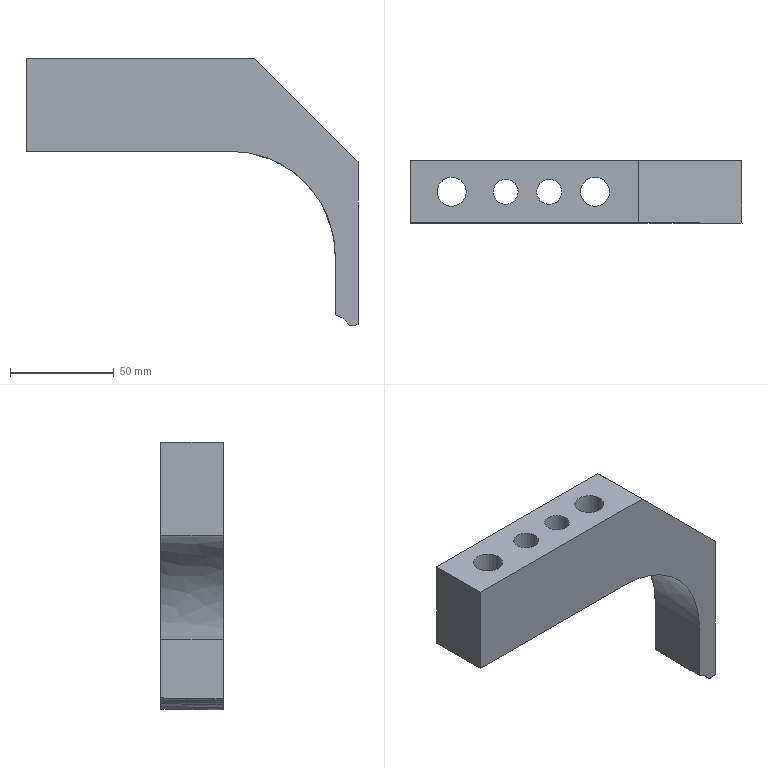Part | NX | features solid 2 | 1 solid | 25 faces | box 160 x 30.001 x 129.104 mm | volume 191101 mm3 | spline 11 | plane 8 | cylinder 6 | commonest cylinder face diameters 12 x2 14 x2 20 x2
STEP:
#1=CARTESIAN_POINT('',(680.804,105.,-27.89));
#2=VERTEX_POINT('',#1);
#3=CARTESIAN_POINT('',(684.074,105.,-28.985));
#4=VERTEX_POINT('',#3);
#5=CARTESIAN_POINT('',(680.804,105.,-27.89));
#6=CARTESIAN_POINT('',(681.537,105.,-28.885));
#7=CARTESIAN_POINT('',(682.89,105.,-29.338));
#8=CARTESIAN_POINT('',(684.074,105.,-28.985));
#9=B_SPLINE_CURVE_WITH_KNOTS('',3,(#5,#6,#7,#8),.UNSPECIFIED.,.F.,.F.,(4,4),(0.,0.003653),.UNSPECIFIED.);
#10=EDGE_CURVE('',#2,#4,#9,.T.);
#11=ORIENTED_EDGE('',*,*,#10,.T.);
#12=CARTESIAN_POINT('',(685.886,105.,-28.443));
#13=VERTEX_POINT('',#12);
#14=CARTESIAN_POINT('',(684.074,105.,-28.985));
#15=CARTESIAN_POINT('',(684.678,105.,-28.805));
#16=CARTESIAN_POINT('',(685.282,105.,-28.624));
#17=CARTESIAN_POINT('',(685.886,105.,-28.443));
#18=B_SPLINE_CURVE_WITH_KNOTS('',3,(#14,#15,#16,#17),.UNSPECIFIED.,.F.,.F.,(4,4),(0.01804,0.01993),.UNSPECIFIED.);
#19=EDGE_CURVE('',#4,#13,#18,.T.);
#20=ORIENTED_EDGE('',*,*,#19,.T.);
#21=CARTESIAN_POINT('',(685.886,105.,50.));
#22=VERTEX_POINT('',#21);
#23=CARTESIAN_POINT('',(685.886,105.,30.));
#24=DIRECTION('',(0.,0.,-1.));
#25=VECTOR('',#24,1000.);
#26=LINE('',#23,#25);
#27=EDGE_CURVE('',#22,#13,#26,.T.);
#28=ORIENTED_EDGE('',*,*,#27,.F.);
#29=CARTESIAN_POINT('',(635.885,105.,100.));
#30=VERTEX_POINT('',#29);
#31=CARTESIAN_POINT('',(685.885,105.,50.));
#32=CARTESIAN_POINT('',(669.219,105.,66.667));
#33=CARTESIAN_POINT('',(652.552,105.,83.333));
#34=CARTESIAN_POINT('',(635.885,105.,100.));
#35=B_SPLINE_CURVE_WITH_KNOTS('',3,(#31,#32,#33,#34),.UNSPECIFIED.,.F.,.F.,(4,4),(0.,1.),.UNSPECIFIED.);
#36=EDGE_CURVE('',#22,#30,#35,.T.);
#37=ORIENTED_EDGE('',*,*,#36,.T.);
#38=CARTESIAN_POINT('',(525.886,105.,100.));
#39=VERTEX_POINT('',#38);
#40=CARTESIAN_POINT('',(664.886,105.,100.));
#41=DIRECTION('',(-1.,0.,0.));
#42=VECTOR('',#41,1000.);
#43=LINE('',#40,#42);
#44=EDGE_CURVE('',#30,#39,#43,.T.);
#45=ORIENTED_EDGE('',*,*,#44,.T.);
#46=CARTESIAN_POINT('',(525.886,105.,55.));
#47=VERTEX_POINT('',#46);
#48=CARTESIAN_POINT('',(525.886,105.,-200.));
#49=DIRECTION('',(0.,0.,1.));
#50=VECTOR('',#49,1000.);
#51=LINE('',#48,#50);
#52=EDGE_CURVE('',#47,#39,#51,.T.);
#53=ORIENTED_EDGE('',*,*,#52,.F.);
#54=CARTESIAN_POINT('',(624.886,105.,55.));
#55=VERTEX_POINT('',#54);
#56=CARTESIAN_POINT('',(531.,105.,55.));
#57=DIRECTION('',(-1.,0.,0.));
#58=VECTOR('',#57,1000.);
#59=LINE('',#56,#58);
#60=EDGE_CURVE('',#55,#47,#59,.T.);
#61=ORIENTED_EDGE('',*,*,#60,.F.);
#62=CARTESIAN_POINT('',(674.886,105.,5.));
#63=VERTEX_POINT('',#62);
#64=CARTESIAN_POINT('',(624.886,105.,55.));
#65=CARTESIAN_POINT('',(628.187,105.,55.));
#66=CARTESIAN_POINT('',(634.66,105.,54.363));
#67=CARTESIAN_POINT('',(644.167,105.,51.481));
#68=CARTESIAN_POINT('',(652.789,105.,46.876));
#69=CARTESIAN_POINT('',(660.473,105.,40.581));
#70=CARTESIAN_POINT('',(666.689,105.,33.01));
#71=CARTESIAN_POINT('',(672.922,105.,21.389));
#72=CARTESIAN_POINT('',(674.886,105.,11.603));
#73=CARTESIAN_POINT('',(674.886,105.,5.));
#74=B_SPLINE_CURVE_WITH_KNOTS('',3,(#64,#65,#66,#67,#68,#69,#70,#71,#72,#73),.UNSPECIFIED.,.F.,.F.,(4,1,1,1,1,1,1,4),(0.,0.009763,0.01953,0.02929,0.03905,0.04882,0.05858,0.07811),.UNSPECIFIED.);
#75=EDGE_CURVE('',#55,#63,#74,.T.);
#76=ORIENTED_EDGE('',*,*,#75,.T.);
#77=CARTESIAN_POINT('',(674.886,105.,-23.672));
#78=VERTEX_POINT('',#77);
#79=CARTESIAN_POINT('',(674.886,105.,44.358));
#80=DIRECTION('',(0.,0.,-1.));
#81=VECTOR('',#80,1000.);
#82=LINE('',#79,#81);
#83=EDGE_CURVE('',#63,#78,#82,.T.);
#84=ORIENTED_EDGE('',*,*,#83,.T.);
#85=CARTESIAN_POINT('',(677.15,105.,-24.654));
#86=VERTEX_POINT('',#85);
#87=CARTESIAN_POINT('',(674.886,105.,-23.672));
#88=CARTESIAN_POINT('',(675.59,105.,-24.088));
#89=CARTESIAN_POINT('',(676.354,105.,-24.42));
#90=CARTESIAN_POINT('',(677.15,105.,-24.654));
#91=B_SPLINE_CURVE_WITH_KNOTS('',3,(#87,#88,#89,#90),.UNSPECIFIED.,.F.,.F.,(4,4),(0.008596,0.01105),.UNSPECIFIED.);
#92=EDGE_CURVE('',#78,#86,#91,.T.);
#93=ORIENTED_EDGE('',*,*,#92,.T.);
#94=CARTESIAN_POINT('',(679.767,105.,-26.484));
#95=VERTEX_POINT('',#94);
#96=CARTESIAN_POINT('',(677.136,105.,-24.65));
#97=CARTESIAN_POINT('',(678.187,105.,-24.955));
#98=CARTESIAN_POINT('',(679.117,105.,-25.604));
#99=CARTESIAN_POINT('',(679.767,105.,-26.484));
#100=B_SPLINE_CURVE_WITH_KNOTS('',3,(#96,#97,#98,#99),.UNSPECIFIED.,.F.,.F.,(4,4),(0.,0.00327),.UNSPECIFIED.);
#101=EDGE_CURVE('',#86,#95,#100,.T.);
#102=ORIENTED_EDGE('',*,*,#101,.T.);
#103=CARTESIAN_POINT('',(679.76,105.,-26.476));
#104=CARTESIAN_POINT('',(680.108,105.,-26.947));
#105=CARTESIAN_POINT('',(680.456,105.,-27.419));
#106=CARTESIAN_POINT('',(680.804,105.,-27.89));
#107=B_SPLINE_CURVE_WITH_KNOTS('',3,(#103,#104,#105,#106),.UNSPECIFIED.,.F.,.F.,(4,4),(0.,0.001758),.UNSPECIFIED.);
#108=EDGE_CURVE('',#95,#2,#107,.T.);
#109=ORIENTED_EDGE('',*,*,#108,.T.);
#110=EDGE_LOOP('',(#11,#20,#28,#37,#45,#53,#61,#76,#84,#93,#102,#109));
#111=FACE_BOUND('',#110,.T.);
#112=CARTESIAN_POINT('',(664.886,105.,-200.));
#113=DIRECTION('',(0.,1.,0.));
#114=DIRECTION('',(0.,0.,1.));
#115=AXIS2_PLACEMENT_3D('',#112,#113,#114);
#116=PLANE('',#115);
#117=ADVANCED_FACE('',(#111),#116,.F.);
#118=CARTESIAN_POINT('',(635.875,135.,100.));
#119=VERTEX_POINT('',#118);
#120=CARTESIAN_POINT('',(525.886,135.,100.));
#121=VERTEX_POINT('',#120);
#122=CARTESIAN_POINT('',(664.883,135.,100.));
#123=DIRECTION('',(-1.,0.,0.));
#124=VECTOR('',#123,1000.);
#125=LINE('',#122,#124);
#126=EDGE_CURVE('',#119,#121,#125,.T.);
#127=ORIENTED_EDGE('',*,*,#126,.F.);
#128=CARTESIAN_POINT('',(685.179,135.,50.704));
#129=VERTEX_POINT('',#128);
#130=CARTESIAN_POINT('',(635.884,135.,100.));
#131=CARTESIAN_POINT('',(652.316,135.,83.568));
#132=CARTESIAN_POINT('',(668.747,135.,67.136));
#133=CARTESIAN_POINT('',(685.179,135.,50.704));
#134=B_SPLINE_CURVE_WITH_KNOTS('',3,(#130,#131,#132,#133),.UNSPECIFIED.,.F.,.F.,(4,4),(0.,1.),.UNSPECIFIED.);
#135=EDGE_CURVE('',#119,#129,#134,.T.);
#136=ORIENTED_EDGE('',*,*,#135,.T.);
#137=CARTESIAN_POINT('',(684.884,135.,30.));
#138=VERTEX_POINT('',#137);
#139=CARTESIAN_POINT('',(685.179,135.,50.704));
#140=CARTESIAN_POINT('',(685.081,135.,43.803));
#141=CARTESIAN_POINT('',(684.982,135.,36.901));
#142=CARTESIAN_POINT('',(684.884,135.,30.));
#143=B_SPLINE_CURVE_WITH_KNOTS('',3,(#139,#140,#141,#142),.UNSPECIFIED.,.F.,.F.,(4,4),(0.7042,1.),.UNSPECIFIED.);
#144=EDGE_CURVE('',#129,#138,#143,.T.);
#145=ORIENTED_EDGE('',*,*,#144,.T.);
#146=CARTESIAN_POINT('',(684.317,135.,30.));
#147=VERTEX_POINT('',#146);
#148=CARTESIAN_POINT('',(684.884,135.,30.));
#149=CARTESIAN_POINT('',(684.695,135.,30.));
#150=CARTESIAN_POINT('',(684.506,135.,30.));
#151=CARTESIAN_POINT('',(684.317,135.,30.));
#152=B_SPLINE_CURVE_WITH_KNOTS('',3,(#148,#149,#150,#151),.UNSPECIFIED.,.F.,.F.,(4,4),(0.,1.),.UNSPECIFIED.);
#153=EDGE_CURVE('',#138,#147,#152,.T.);
#154=ORIENTED_EDGE('',*,*,#153,.T.);
#155=CARTESIAN_POINT('',(674.884,135.001,30.));
#156=VERTEX_POINT('',#155);
#157=CARTESIAN_POINT('',(684.317,135.,30.));
#158=CARTESIAN_POINT('',(681.172,135.,30.));
#159=CARTESIAN_POINT('',(678.028,135.,30.));
#160=CARTESIAN_POINT('',(674.884,135.,30.));
#161=B_SPLINE_CURVE_WITH_KNOTS('',3,(#157,#158,#159,#160),.UNSPECIFIED.,.F.,.F.,(4,4),(0.,1.),.UNSPECIFIED.);
#162=EDGE_CURVE('',#147,#156,#161,.T.);
#163=ORIENTED_EDGE('',*,*,#162,.T.);
#164=CARTESIAN_POINT('',(668.185,135.001,30.));
#165=VERTEX_POINT('',#164);
#166=CARTESIAN_POINT('',(674.884,135.,30.));
#167=CARTESIAN_POINT('',(672.651,135.,30.));
#168=CARTESIAN_POINT('',(670.418,135.,30.));
#169=CARTESIAN_POINT('',(668.185,135.,30.));
#170=B_SPLINE_CURVE_WITH_KNOTS('',3,(#166,#167,#168,#169),.UNSPECIFIED.,.F.,.F.,(4,4),(0.,1.),.UNSPECIFIED.);
#171=EDGE_CURVE('',#156,#165,#170,.T.);
#172=ORIENTED_EDGE('',*,*,#171,.T.);
#173=CARTESIAN_POINT('',(624.884,135.,55.));
#174=VERTEX_POINT('',#173);
#175=CARTESIAN_POINT('',(668.185,135.,30.));
#176=CARTESIAN_POINT('',(665.981,135.,33.818));
#177=CARTESIAN_POINT('',(662.018,135.,38.982));
#178=CARTESIAN_POINT('',(655.372,135.,44.812));
#179=CARTESIAN_POINT('',(649.946,135.,48.428));
#180=CARTESIAN_POINT('',(644.065,135.,51.332));
#181=CARTESIAN_POINT('',(635.725,135.,54.151));
#182=CARTESIAN_POINT('',(629.292,135.,55.));
#183=CARTESIAN_POINT('',(624.884,135.,55.));
#184=B_SPLINE_CURVE_WITH_KNOTS('',3,(#175,#176,#177,#178,#179,#180,#181,#182,#183),.UNSPECIFIED.,.F.,.F.,(4,1,1,1,1,1,4),(0.,0.01304,0.01956,0.02608,0.03259,0.03911,0.05215),.UNSPECIFIED.);
#185=EDGE_CURVE('',#165,#174,#184,.T.);
#186=ORIENTED_EDGE('',*,*,#185,.T.);
#187=CARTESIAN_POINT('',(525.886,135.,55.));
#188=VERTEX_POINT('',#187);
#189=CARTESIAN_POINT('',(664.883,135.,55.));
#190=DIRECTION('',(-1.,0.,0.));
#191=VECTOR('',#190,1000.);
#192=LINE('',#189,#191);
#193=EDGE_CURVE('',#174,#188,#192,.T.);
#194=ORIENTED_EDGE('',*,*,#193,.T.);
#195=CARTESIAN_POINT('',(525.886,135.,-200.));
#196=DIRECTION('',(0.,0.,1.));
#197=VECTOR('',#196,1000.);
#198=LINE('',#195,#197);
#199=EDGE_CURVE('',#188,#121,#198,.T.);
#200=ORIENTED_EDGE('',*,*,#199,.T.);
#201=EDGE_LOOP('',(#127,#136,#145,#154,#163,#172,#186,#194,#200));
#202=FACE_BOUND('',#201,.T.);
#203=CARTESIAN_POINT('',(664.883,135.,-200.));
#204=DIRECTION('',(0.,1.,0.));
#205=DIRECTION('',(0.,0.,1.));
#206=AXIS2_PLACEMENT_3D('',#203,#204,#205);
#207=PLANE('',#206);
#208=ADVANCED_FACE('',(#202),#207,.T.);
#209=CARTESIAN_POINT('',(525.886,135.,55.));
#210=DIRECTION('',(0.,-1.,0.));
#211=VECTOR('',#210,1000.);
#212=LINE('',#209,#211);
#213=EDGE_CURVE('',#188,#47,#212,.T.);
#214=ORIENTED_EDGE('',*,*,#213,.T.);
#215=ORIENTED_EDGE('',*,*,#52,.T.);
#216=CARTESIAN_POINT('',(525.886,175.,100.));
#217=DIRECTION('',(0.,-1.,0.));
#218=VECTOR('',#217,1000.);
#219=LINE('',#216,#218);
#220=EDGE_CURVE('',#121,#39,#219,.T.);
#221=ORIENTED_EDGE('',*,*,#220,.F.);
#222=ORIENTED_EDGE('',*,*,#199,.F.);
#223=EDGE_LOOP('',(#214,#215,#221,#222));
#224=FACE_BOUND('',#223,.T.);
#225=CARTESIAN_POINT('',(525.886,175.,75.));
#226=DIRECTION('',(-1.,0.,0.));
#227=DIRECTION('',(0.,0.,1.));
#228=AXIS2_PLACEMENT_3D('',#225,#226,#227);
#229=PLANE('',#228);
#230=ADVANCED_FACE('',(#224),#229,.T.);
#231=CARTESIAN_POINT('',(587.,120.,100.));
#232=VERTEX_POINT('',#231);
#233=CARTESIAN_POINT('',(593.,120.,100.));
#234=DIRECTION('',(0.,0.,-1.));
#235=DIRECTION('',(-1.,0.,0.));
#236=AXIS2_PLACEMENT_3D('',#233,#234,#235);
#237=CIRCLE('',#236,6.);
#238=EDGE_CURVE('',#232,#232,#237,.T.);
#239=ORIENTED_EDGE('',*,*,#238,.T.);
#240=EDGE_LOOP('',(#239));
#241=FACE_BOUND('',#240,.T.);
#242=CARTESIAN_POINT('',(566.,120.,100.));
#243=VERTEX_POINT('',#242);
#244=CARTESIAN_POINT('',(572.,120.,100.));
#245=DIRECTION('',(0.,0.,-1.));
#246=DIRECTION('',(-1.,0.,0.));
#247=AXIS2_PLACEMENT_3D('',#244,#245,#246);
#248=CIRCLE('',#247,6.);
#249=EDGE_CURVE('',#243,#243,#248,.T.);
#250=ORIENTED_EDGE('',*,*,#249,.T.);
#251=EDGE_LOOP('',(#250));
#252=FACE_BOUND('',#251,.T.);
#253=CARTESIAN_POINT('',(608.,120.,100.));
#254=VERTEX_POINT('',#253);
#255=CARTESIAN_POINT('',(615.,120.,100.));
#256=DIRECTION('',(0.,0.,-1.));
#257=DIRECTION('',(-1.,0.,0.));
#258=AXIS2_PLACEMENT_3D('',#255,#256,#257);
#259=CIRCLE('',#258,7.);
#260=EDGE_CURVE('',#254,#254,#259,.T.);
#261=ORIENTED_EDGE('',*,*,#260,.T.);
#262=EDGE_LOOP('',(#261));
#263=FACE_BOUND('',#262,.T.);
#264=CARTESIAN_POINT('',(539.,120.,100.));
#265=VERTEX_POINT('',#264);
#266=CARTESIAN_POINT('',(546.,120.,100.));
#267=DIRECTION('',(0.,0.,-1.));
#268=DIRECTION('',(-1.,0.,0.));
#269=AXIS2_PLACEMENT_3D('',#266,#267,#268);
#270=CIRCLE('',#269,7.);
#271=EDGE_CURVE('',#265,#265,#270,.T.);
#272=ORIENTED_EDGE('',*,*,#271,.T.);
#273=EDGE_LOOP('',(#272));
#274=FACE_BOUND('',#273,.T.);
#275=ORIENTED_EDGE('',*,*,#44,.F.);
#276=CARTESIAN_POINT('',(635.885,105.,100.));
#277=CARTESIAN_POINT('',(635.885,115.,100.));
#278=CARTESIAN_POINT('',(635.884,125.,100.));
#279=CARTESIAN_POINT('',(635.884,135.,100.));
#280=B_SPLINE_CURVE_WITH_KNOTS('',3,(#276,#277,#278,#279),.UNSPECIFIED.,.F.,.F.,(4,4),(0.,1.),.UNSPECIFIED.);
#281=EDGE_CURVE('',#30,#119,#280,.T.);
#282=ORIENTED_EDGE('',*,*,#281,.T.);
#283=ORIENTED_EDGE('',*,*,#126,.T.);
#284=ORIENTED_EDGE('',*,*,#220,.T.);
#285=EDGE_LOOP('',(#275,#282,#283,#284));
#286=FACE_BOUND('',#285,.T.);
#287=CARTESIAN_POINT('',(561.,60.,100.));
#288=DIRECTION('',(0.,0.,-1.));
#289=DIRECTION('',(-1.,0.,0.));
#290=AXIS2_PLACEMENT_3D('',#287,#288,#289);
#291=PLANE('',#290);
#292=ADVANCED_FACE('',(#241,#252,#263,#274,#286),#291,.F.);
#293=CARTESIAN_POINT('',(553.,120.,75.));
#294=VERTEX_POINT('',#293);
#295=CARTESIAN_POINT('',(546.,120.,75.));
#296=DIRECTION('',(0.,0.,1.));
#297=DIRECTION('',(1.,0.,0.));
#298=AXIS2_PLACEMENT_3D('',#295,#296,#297);
#299=CIRCLE('',#298,7.);
#300=EDGE_CURVE('',#294,#294,#299,.T.);
#301=ORIENTED_EDGE('',*,*,#300,.F.);
#302=EDGE_LOOP('',(#301));
#303=FACE_BOUND('',#302,.T.);
#304=ORIENTED_EDGE('',*,*,#271,.F.);
#305=EDGE_LOOP('',(#304));
#306=FACE_BOUND('',#305,.T.);
#307=CARTESIAN_POINT('',(546.,120.,75.));
#308=DIRECTION('',(0.,0.,1.));
#309=DIRECTION('',(-1.,0.,0.));
#310=AXIS2_PLACEMENT_3D('',#307,#308,#309);
#311=CYLINDRICAL_SURFACE('',#310,7.);
#312=ADVANCED_FACE('',(#303,#306),#311,.F.);
#313=ORIENTED_EDGE('',*,*,#300,.T.);
#314=EDGE_LOOP('',(#313));
#315=FACE_BOUND('',#314,.T.);
#316=CARTESIAN_POINT('',(556.,120.,75.));
#317=VERTEX_POINT('',#316);
#318=CARTESIAN_POINT('',(546.,120.,75.));
#319=DIRECTION('',(0.,0.,-1.));
#320=DIRECTION('',(1.,0.,0.));
#321=AXIS2_PLACEMENT_3D('',#318,#319,#320);
#322=CIRCLE('',#321,10.);
#323=EDGE_CURVE('',#317,#317,#322,.T.);
#324=ORIENTED_EDGE('',*,*,#323,.T.);
#325=EDGE_LOOP('',(#324));
#326=FACE_BOUND('',#325,.T.);
#327=CARTESIAN_POINT('',(546.,120.,75.));
#328=DIRECTION('',(0.,0.,1.));
#329=DIRECTION('',(-1.,0.,0.));
#330=AXIS2_PLACEMENT_3D('',#327,#328,#329);
#331=PLANE('',#330);
#332=ADVANCED_FACE('',(#315,#326),#331,.F.);
#333=CARTESIAN_POINT('',(556.,120.,55.));
#334=VERTEX_POINT('',#333);
#335=CARTESIAN_POINT('',(546.,120.,55.));
#336=DIRECTION('',(0.,0.,1.));
#337=DIRECTION('',(1.,0.,0.));
#338=AXIS2_PLACEMENT_3D('',#335,#336,#337);
#339=CIRCLE('',#338,10.);
#340=EDGE_CURVE('',#334,#334,#339,.F.);
#341=ORIENTED_EDGE('',*,*,#340,.T.);
#342=EDGE_LOOP('',(#341));
#343=FACE_BOUND('',#342,.T.);
#344=ORIENTED_EDGE('',*,*,#323,.F.);
#345=EDGE_LOOP('',(#344));
#346=FACE_BOUND('',#345,.T.);
#347=CARTESIAN_POINT('',(546.,120.,75.));
#348=DIRECTION('',(0.,0.,-1.));
#349=DIRECTION('',(1.,0.,0.));
#350=AXIS2_PLACEMENT_3D('',#347,#348,#349);
#351=CYLINDRICAL_SURFACE('',#350,10.);
#352=ADVANCED_FACE('',(#343,#346),#351,.F.);
#353=CARTESIAN_POINT('',(622.,120.,75.));
#354=VERTEX_POINT('',#353);
#355=CARTESIAN_POINT('',(615.,120.,75.));
#356=DIRECTION('',(0.,0.,1.));
#357=DIRECTION('',(1.,0.,0.));
#358=AXIS2_PLACEMENT_3D('',#355,#356,#357);
#359=CIRCLE('',#358,7.);
#360=EDGE_CURVE('',#354,#354,#359,.T.);
#361=ORIENTED_EDGE('',*,*,#360,.F.);
#362=EDGE_LOOP('',(#361));
#363=FACE_BOUND('',#362,.T.);
#364=ORIENTED_EDGE('',*,*,#260,.F.);
#365=EDGE_LOOP('',(#364));
#366=FACE_BOUND('',#365,.T.);
#367=CARTESIAN_POINT('',(615.,120.,72.));
#368=DIRECTION('',(0.,0.,1.));
#369=DIRECTION('',(-1.,0.,0.));
#370=AXIS2_PLACEMENT_3D('',#367,#368,#369);
#371=CYLINDRICAL_SURFACE('',#370,7.);
#372=ADVANCED_FACE('',(#363,#366),#371,.F.);
#373=CARTESIAN_POINT('',(624.883,118.475,55.));
#374=VERTEX_POINT('',#373);
#375=CARTESIAN_POINT('',(624.883,121.526,55.));
#376=VERTEX_POINT('',#375);
#377=CARTESIAN_POINT('',(615.,120.,55.));
#378=DIRECTION('',(0.,0.,1.));
#379=DIRECTION('',(1.,0.,0.));
#380=AXIS2_PLACEMENT_3D('',#377,#378,#379);
#381=CIRCLE('',#380,10.);
#382=EDGE_CURVE('',#374,#376,#381,.F.);
#383=ORIENTED_EDGE('',*,*,#382,.T.);
#384=CARTESIAN_POINT('',(624.883,118.475,55.));
#385=CARTESIAN_POINT('',(625.038,119.479,55.));
#386=CARTESIAN_POINT('',(625.038,120.522,55.));
#387=CARTESIAN_POINT('',(624.883,121.526,55.));
#388=B_SPLINE_CURVE_WITH_KNOTS('',3,(#384,#385,#386,#387),.UNSPECIFIED.,.F.,.F.,(4,4),(0.001833,0.00488),.UNSPECIFIED.);
#389=EDGE_CURVE('',#376,#374,#388,.F.);
#390=ORIENTED_EDGE('',*,*,#389,.T.);
#391=EDGE_LOOP('',(#383,#390));
#392=FACE_BOUND('',#391,.T.);
#393=CARTESIAN_POINT('',(625.,120.,75.));
#394=VERTEX_POINT('',#393);
#395=CARTESIAN_POINT('',(615.,120.,75.));
#396=DIRECTION('',(0.,0.,1.));
#397=DIRECTION('',(1.,0.,0.));
#398=AXIS2_PLACEMENT_3D('',#395,#396,#397);
#399=CIRCLE('',#398,10.);
#400=EDGE_CURVE('',#394,#394,#399,.F.);
#401=ORIENTED_EDGE('',*,*,#400,.F.);
#402=EDGE_LOOP('',(#401));
#403=FACE_BOUND('',#402,.T.);
#404=CARTESIAN_POINT('',(615.,120.,72.));
#405=DIRECTION('',(0.,0.,-1.));
#406=DIRECTION('',(1.,0.,0.));
#407=AXIS2_PLACEMENT_3D('',#404,#405,#406);
#408=CYLINDRICAL_SURFACE('',#407,10.);
#409=ADVANCED_FACE('',(#392,#403),#408,.F.);
#410=ORIENTED_EDGE('',*,*,#360,.T.);
#411=EDGE_LOOP('',(#410));
#412=FACE_BOUND('',#411,.T.);
#413=ORIENTED_EDGE('',*,*,#400,.T.);
#414=EDGE_LOOP('',(#413));
#415=FACE_BOUND('',#414,.T.);
#416=CARTESIAN_POINT('',(615.,120.,75.));
#417=DIRECTION('',(0.,0.,1.));
#418=DIRECTION('',(-1.,0.,0.));
#419=AXIS2_PLACEMENT_3D('',#416,#417,#418);
#420=PLANE('',#419);
#421=ADVANCED_FACE('',(#412,#415),#420,.F.);
#422=CARTESIAN_POINT('',(587.,120.,55.));
#423=VERTEX_POINT('',#422);
#424=CARTESIAN_POINT('',(593.,120.,55.));
#425=DIRECTION('',(0.,0.,-1.));
#426=DIRECTION('',(-1.,0.,0.));
#427=AXIS2_PLACEMENT_3D('',#424,#425,#426);
#428=CIRCLE('',#427,6.);
#429=EDGE_CURVE('',#423,#423,#428,.T.);
#430=ORIENTED_EDGE('',*,*,#429,.F.);
#431=EDGE_LOOP('',(#430));
#432=FACE_BOUND('',#431,.T.);
#433=CARTESIAN_POINT('',(566.,120.,55.));
#434=VERTEX_POINT('',#433);
#435=CARTESIAN_POINT('',(572.,120.,55.));
#436=DIRECTION('',(0.,0.,-1.));
#437=DIRECTION('',(-1.,0.,0.));
#438=AXIS2_PLACEMENT_3D('',#435,#436,#437);
#439=CIRCLE('',#438,6.);
#440=EDGE_CURVE('',#434,#434,#439,.T.);
#441=ORIENTED_EDGE('',*,*,#440,.F.);
#442=EDGE_LOOP('',(#441));
#443=FACE_BOUND('',#442,.T.);
#444=ORIENTED_EDGE('',*,*,#193,.F.);
#445=CARTESIAN_POINT('',(624.884,135.,55.));
#446=CARTESIAN_POINT('',(624.883,130.509,55.));
#447=CARTESIAN_POINT('',(624.883,126.017,55.));
#448=CARTESIAN_POINT('',(624.883,121.526,55.));
#449=B_SPLINE_CURVE_WITH_KNOTS('',3,(#445,#446,#447,#448),.UNSPECIFIED.,.F.,.F.,(4,4),(0.,0.01347),.UNSPECIFIED.);
#450=EDGE_CURVE('',#174,#376,#449,.T.);
#451=ORIENTED_EDGE('',*,*,#450,.T.);
#452=ORIENTED_EDGE('',*,*,#382,.F.);
#453=CARTESIAN_POINT('',(624.883,118.475,55.));
#454=CARTESIAN_POINT('',(624.883,113.983,55.));
#455=CARTESIAN_POINT('',(624.884,109.492,55.));
#456=CARTESIAN_POINT('',(624.886,105.,55.));
#457=B_SPLINE_CURVE_WITH_KNOTS('',3,(#453,#454,#455,#456),.UNSPECIFIED.,.F.,.F.,(4,4),(0.01653,0.03),.UNSPECIFIED.);
#458=EDGE_CURVE('',#374,#55,#457,.T.);
#459=ORIENTED_EDGE('',*,*,#458,.T.);
#460=ORIENTED_EDGE('',*,*,#60,.T.);
#461=ORIENTED_EDGE('',*,*,#213,.F.);
#462=EDGE_LOOP('',(#444,#451,#452,#459,#460,#461));
#463=FACE_BOUND('',#462,.T.);
#464=ORIENTED_EDGE('',*,*,#340,.F.);
#465=EDGE_LOOP('',(#464));
#466=FACE_BOUND('',#465,.T.);
#467=CARTESIAN_POINT('',(531.,135.,55.));
#468=DIRECTION('',(0.,0.,1.));
#469=DIRECTION('',(0.,-1.,0.));
#470=AXIS2_PLACEMENT_3D('',#467,#468,#469);
#471=PLANE('',#470);
#472=ADVANCED_FACE('',(#432,#443,#463,#466),#471,.F.);
#473=ORIENTED_EDGE('',*,*,#249,.F.);
#474=EDGE_LOOP('',(#473));
#475=FACE_BOUND('',#474,.T.);
#476=ORIENTED_EDGE('',*,*,#440,.T.);
#477=EDGE_LOOP('',(#476));
#478=FACE_BOUND('',#477,.T.);
#479=CARTESIAN_POINT('',(572.,120.,105.));
#480=DIRECTION('',(0.,0.,-1.));
#481=DIRECTION('',(-1.,0.,0.));
#482=AXIS2_PLACEMENT_3D('',#479,#480,#481);
#483=CYLINDRICAL_SURFACE('',#482,6.);
#484=ADVANCED_FACE('',(#475,#478),#483,.F.);
#485=ORIENTED_EDGE('',*,*,#238,.F.);
#486=EDGE_LOOP('',(#485));
#487=FACE_BOUND('',#486,.T.);
#488=ORIENTED_EDGE('',*,*,#429,.T.);
#489=EDGE_LOOP('',(#488));
#490=FACE_BOUND('',#489,.T.);
#491=CARTESIAN_POINT('',(593.,120.,105.));
#492=DIRECTION('',(0.,0.,-1.));
#493=DIRECTION('',(-1.,0.,0.));
#494=AXIS2_PLACEMENT_3D('',#491,#492,#493);
#495=CYLINDRICAL_SURFACE('',#494,6.);
#496=ADVANCED_FACE('',(#487,#490),#495,.F.);
#497=CARTESIAN_POINT('',(674.884,135.001,-23.321));
#498=VERTEX_POINT('',#497);
#499=CARTESIAN_POINT('',(674.883,122.627,-23.464));
#500=VERTEX_POINT('',#499);
#501=CARTESIAN_POINT('',(674.884,135.001,-23.321));
#502=CARTESIAN_POINT('',(674.883,130.876,-23.369));
#503=CARTESIAN_POINT('',(674.883,126.752,-23.415));
#504=CARTESIAN_POINT('',(674.883,122.627,-23.464));
#505=B_SPLINE_CURVE_WITH_KNOTS('',3,(#501,#502,#503,#504),.UNSPECIFIED.,.F.,.F.,(4,4),(0.,0.01237),.UNSPECIFIED.);
#506=EDGE_CURVE('',#498,#500,#505,.T.);
#507=ORIENTED_EDGE('',*,*,#506,.T.);
#508=CARTESIAN_POINT('',(674.883,122.627,-23.464));
#509=CARTESIAN_POINT('',(674.883,116.751,-23.533));
#510=CARTESIAN_POINT('',(674.884,110.876,-23.603));
#511=CARTESIAN_POINT('',(674.886,105.,-23.672));
#512=B_SPLINE_CURVE_WITH_KNOTS('',3,(#508,#509,#510,#511),.UNSPECIFIED.,.F.,.F.,(4,4),(0.,0.01763),.UNSPECIFIED.);
#513=EDGE_CURVE('',#500,#78,#512,.T.);
#514=ORIENTED_EDGE('',*,*,#513,.T.);
#515=ORIENTED_EDGE('',*,*,#83,.F.);
#516=CARTESIAN_POINT('',(674.884,135.001,5.));
#517=VERTEX_POINT('',#516);
#518=CARTESIAN_POINT('',(674.886,105.,5.));
#519=CARTESIAN_POINT('',(674.882,115.,5.));
#520=CARTESIAN_POINT('',(674.883,125.001,5.));
#521=CARTESIAN_POINT('',(674.884,135.001,5.));
#522=B_SPLINE_CURVE_WITH_KNOTS('',3,(#518,#519,#520,#521),.UNSPECIFIED.,.F.,.F.,(4,4),(0.,0.03),.UNSPECIFIED.);
#523=EDGE_CURVE('',#63,#517,#522,.T.);
#524=ORIENTED_EDGE('',*,*,#523,.T.);
#525=CARTESIAN_POINT('',(674.884,135.001,30.));
#526=DIRECTION('',(0.,0.,-1.));
#527=VECTOR('',#526,1000.);
#528=LINE('',#525,#527);
#529=EDGE_CURVE('',#517,#498,#528,.T.);
#530=ORIENTED_EDGE('',*,*,#529,.T.);
#531=EDGE_LOOP('',(#507,#514,#515,#524,#530));
#532=FACE_BOUND('',#531,.T.);
#533=CARTESIAN_POINT('',(674.884,135.001,5.));
#534=CARTESIAN_POINT('',(674.884,135.001,-23.844));
#535=CARTESIAN_POINT('',(674.883,125.002,5.));
#536=CARTESIAN_POINT('',(674.883,125.002,-23.844));
#537=CARTESIAN_POINT('',(674.882,115.001,5.));
#538=CARTESIAN_POINT('',(674.882,115.001,-23.844));
#539=CARTESIAN_POINT('',(674.886,105.,5.));
#540=CARTESIAN_POINT('',(674.886,105.,-23.844));
#541=B_SPLINE_SURFACE_WITH_KNOTS('',3,1,((#533,#534),(#535,#536),(#537,#538),(#539,#540)),.SURF_OF_LINEAR_EXTRUSION.,.F.,.F.,.F.,(4,4),(2,2),(0.,0.9999),(0.,1.),.PIECEWISE_BEZIER_KNOTS.);
#542=ADVANCED_FACE('',(#532),#541,.F.);
#543=CARTESIAN_POINT('',(684.075,135.,-28.612));
#544=VERTEX_POINT('',#543);
#545=CARTESIAN_POINT('',(685.884,135.,-28.07));
#546=VERTEX_POINT('',#545);
#547=CARTESIAN_POINT('',(684.075,135.,-28.612));
#548=CARTESIAN_POINT('',(684.678,135.,-28.432));
#549=CARTESIAN_POINT('',(685.281,135.,-28.251));
#550=CARTESIAN_POINT('',(685.884,135.,-28.07));
#551=B_SPLINE_CURVE_WITH_KNOTS('',3,(#547,#548,#549,#550),.UNSPECIFIED.,.F.,.F.,(4,4),(0.01663,0.01852),.UNSPECIFIED.);
#552=EDGE_CURVE('',#544,#546,#551,.T.);
#553=ORIENTED_EDGE('',*,*,#552,.F.);
#554=CARTESIAN_POINT('',(680.804,135.,-27.517));
#555=VERTEX_POINT('',#554);
#556=CARTESIAN_POINT('',(680.804,135.,-27.517));
#557=CARTESIAN_POINT('',(681.537,135.,-28.511));
#558=CARTESIAN_POINT('',(682.891,135.,-28.964));
#559=CARTESIAN_POINT('',(684.074,135.,-28.612));
#560=B_SPLINE_CURVE_WITH_KNOTS('',3,(#556,#557,#558,#559),.UNSPECIFIED.,.F.,.F.,(4,4),(0.,0.003653),.UNSPECIFIED.);
#561=EDGE_CURVE('',#555,#544,#560,.T.);
#562=ORIENTED_EDGE('',*,*,#561,.F.);
#563=CARTESIAN_POINT('',(679.774,135.,-26.121));
#564=VERTEX_POINT('',#563);
#565=CARTESIAN_POINT('',(679.776,135.,-26.124));
#566=CARTESIAN_POINT('',(680.119,135.,-26.588));
#567=CARTESIAN_POINT('',(680.461,135.,-27.053));
#568=CARTESIAN_POINT('',(680.804,135.,-27.517));
#569=B_SPLINE_CURVE_WITH_KNOTS('',3,(#565,#566,#567,#568),.UNSPECIFIED.,.F.,.F.,(4,4),(0.00002659,0.001758),.UNSPECIFIED.);
#570=EDGE_CURVE('',#564,#555,#569,.T.);
#571=ORIENTED_EDGE('',*,*,#570,.F.);
#572=CARTESIAN_POINT('',(677.142,135.001,-24.284));
#573=VERTEX_POINT('',#572);
#574=CARTESIAN_POINT('',(677.149,135.001,-24.286));
#575=CARTESIAN_POINT('',(678.198,135.001,-24.593));
#576=CARTESIAN_POINT('',(679.122,135.001,-25.236));
#577=CARTESIAN_POINT('',(679.772,135.,-26.118));
#578=B_SPLINE_CURVE_WITH_KNOTS('',3,(#574,#575,#576,#577),.UNSPECIFIED.,.F.,.F.,(4,4),(0.001293,0.004557),.UNSPECIFIED.);
#579=EDGE_CURVE('',#573,#564,#578,.T.);
#580=ORIENTED_EDGE('',*,*,#579,.F.);
#581=CARTESIAN_POINT('',(674.884,135.001,-23.321));
#582=CARTESIAN_POINT('',(675.585,135.001,-23.728));
#583=CARTESIAN_POINT('',(676.345,135.001,-24.054));
#584=CARTESIAN_POINT('',(677.135,135.001,-24.282));
#585=B_SPLINE_CURVE_WITH_KNOTS('',3,(#581,#582,#583,#584),.UNSPECIFIED.,.F.,.F.,(4,4),(0.008683,0.01112),.UNSPECIFIED.);
#586=EDGE_CURVE('',#498,#573,#585,.T.);
#587=ORIENTED_EDGE('',*,*,#586,.F.);
#588=ORIENTED_EDGE('',*,*,#529,.F.);
#589=CARTESIAN_POINT('',(624.884,135.005,5.));
#590=DIRECTION('',(-0.00008819,-1.,0.));
#591=DIRECTION('',(1.,-0.00008819,0.));
#592=AXIS2_PLACEMENT_3D('',#589,#590,#591);
#593=CIRCLE('',#592,50.);
#594=EDGE_CURVE('',#517,#165,#593,.T.);
#595=ORIENTED_EDGE('',*,*,#594,.T.);
#596=ORIENTED_EDGE('',*,*,#171,.F.);
#597=ORIENTED_EDGE('',*,*,#162,.F.);
#598=ORIENTED_EDGE('',*,*,#153,.F.);
#599=ORIENTED_EDGE('',*,*,#144,.F.);
#600=CARTESIAN_POINT('',(685.884,135.,50.));
#601=VERTEX_POINT('',#600);
#602=CARTESIAN_POINT('',(685.179,135.,50.704));
#603=CARTESIAN_POINT('',(685.414,135.,50.469));
#604=CARTESIAN_POINT('',(685.649,135.,50.235));
#605=CARTESIAN_POINT('',(685.884,135.,50.));
#606=B_SPLINE_CURVE_WITH_KNOTS('',3,(#602,#603,#604,#605),.UNSPECIFIED.,.F.,.F.,(4,4),(0.,1.),.UNSPECIFIED.);
#607=EDGE_CURVE('',#129,#601,#606,.T.);
#608=ORIENTED_EDGE('',*,*,#607,.T.);
#609=CARTESIAN_POINT('',(685.884,135.,30.));
#610=DIRECTION('',(0.,0.,-1.));
#611=VECTOR('',#610,1000.);
#612=LINE('',#609,#611);
#613=EDGE_CURVE('',#601,#546,#612,.T.);
#614=ORIENTED_EDGE('',*,*,#613,.T.);
#615=EDGE_LOOP('',(#553,#562,#571,#580,#587,#588,#595,#596,#597,#598,#599,#608,#614));
#616=FACE_BOUND('',#615,.T.);
#617=CARTESIAN_POINT('',(684.884,135.,30.));
#618=DIRECTION('',(-0.00008819,-1.,0.));
#619=DIRECTION('',(0.,0.,-1.));
#620=AXIS2_PLACEMENT_3D('',#617,#618,#619);
#621=PLANE('',#620);
#622=ADVANCED_FACE('',(#616),#621,.F.);
#623=CARTESIAN_POINT('',(685.884,135.,-28.07));
#624=CARTESIAN_POINT('',(685.883,125.,-28.196));
#625=CARTESIAN_POINT('',(685.882,115.,-28.32));
#626=CARTESIAN_POINT('',(685.886,105.,-28.443));
#627=B_SPLINE_CURVE_WITH_KNOTS('',3,(#623,#624,#625,#626),.UNSPECIFIED.,.F.,.F.,(4,4),(0.,0.03),.UNSPECIFIED.);
#628=EDGE_CURVE('',#546,#13,#627,.T.);
#629=ORIENTED_EDGE('',*,*,#628,.F.);
#630=ORIENTED_EDGE('',*,*,#613,.F.);
#631=CARTESIAN_POINT('',(685.885,105.,50.));
#632=CARTESIAN_POINT('',(685.882,114.999,50.));
#633=CARTESIAN_POINT('',(685.883,124.992,50.));
#634=CARTESIAN_POINT('',(685.884,135.,50.));
#635=B_SPLINE_CURVE_WITH_KNOTS('',3,(#631,#632,#633,#634),.UNSPECIFIED.,.F.,.F.,(4,4),(0.,1.),.UNSPECIFIED.);
#636=EDGE_CURVE('',#601,#22,#635,.F.);
#637=ORIENTED_EDGE('',*,*,#636,.T.);
#638=ORIENTED_EDGE('',*,*,#27,.T.);
#639=EDGE_LOOP('',(#629,#630,#637,#638));
#640=FACE_BOUND('',#639,.T.);
#641=CARTESIAN_POINT('',(685.884,135.,50.));
#642=CARTESIAN_POINT('',(685.884,135.,-28.913));
#643=CARTESIAN_POINT('',(685.883,125.,50.));
#644=CARTESIAN_POINT('',(685.883,125.,-28.913));
#645=CARTESIAN_POINT('',(685.882,115.,50.));
#646=CARTESIAN_POINT('',(685.882,115.,-28.913));
#647=CARTESIAN_POINT('',(685.886,105.,50.));
#648=CARTESIAN_POINT('',(685.886,105.,-28.913));
#649=B_SPLINE_SURFACE_WITH_KNOTS('',3,1,((#641,#642),(#643,#644),(#645,#646),(#647,#648)),.SURF_OF_LINEAR_EXTRUSION.,.F.,.F.,.F.,(4,4),(2,2),(0.,1.),(0.,1.),.PIECEWISE_BEZIER_KNOTS.);
#650=ADVANCED_FACE('',(#640),#649,.T.);
#651=ORIENTED_EDGE('',*,*,#594,.F.);
#652=ORIENTED_EDGE('',*,*,#523,.F.);
#653=ORIENTED_EDGE('',*,*,#75,.F.);
#654=ORIENTED_EDGE('',*,*,#458,.F.);
#655=ORIENTED_EDGE('',*,*,#389,.F.);
#656=ORIENTED_EDGE('',*,*,#450,.F.);
#657=ORIENTED_EDGE('',*,*,#185,.F.);
#658=EDGE_LOOP('',(#651,#652,#653,#654,#655,#656,#657));
#659=FACE_BOUND('',#658,.T.);
#660=CARTESIAN_POINT('',(624.884,135.005,55.));
#661=CARTESIAN_POINT('',(674.884,135.001,55.));
#662=CARTESIAN_POINT('',(674.884,135.001,5.));
#663=CARTESIAN_POINT('',(624.883,124.938,55.));
#664=CARTESIAN_POINT('',(674.883,124.932,55.));
#665=CARTESIAN_POINT('',(674.883,124.932,5.));
#666=CARTESIAN_POINT('',(624.882,114.871,55.));
#667=CARTESIAN_POINT('',(674.882,114.887,55.));
#668=CARTESIAN_POINT('',(674.882,114.887,5.));
#669=CARTESIAN_POINT('',(624.886,104.804,55.));
#670=CARTESIAN_POINT('',(674.886,104.82,55.));
#671=CARTESIAN_POINT('',(674.886,104.82,5.));
#672=(BOUNDED_SURFACE()B_SPLINE_SURFACE(3,2,((#660,#661,#662),(#663,#664,#665),(#666,#667,#668),(#669,#670,#671)),.UNSPECIFIED.,.F.,.F.,.F.)B_SPLINE_SURFACE_WITH_KNOTS((4,4),(3,3),(0.12,0.1502),(0.,1.),.PIECEWISE_BEZIER_KNOTS.)GEOMETRIC_REPRESENTATION_ITEM()RATIONAL_B_SPLINE_SURFACE(((1.,0.7071,1.),(1.,0.7071,1.),(1.,0.7071,1.),(1.,0.7071,1.)))REPRESENTATION_ITEM('')SURFACE());
#673=ADVANCED_FACE('',(#659),#672,.F.);
#674=ORIENTED_EDGE('',*,*,#135,.F.);
#675=ORIENTED_EDGE('',*,*,#281,.F.);
#676=ORIENTED_EDGE('',*,*,#36,.F.);
#677=ORIENTED_EDGE('',*,*,#636,.F.);
#678=ORIENTED_EDGE('',*,*,#607,.F.);
#679=EDGE_LOOP('',(#674,#675,#676,#677,#678));
#680=FACE_BOUND('',#679,.T.);
#681=CARTESIAN_POINT('',(635.886,104.805,100.));
#682=CARTESIAN_POINT('',(635.882,114.871,100.));
#683=CARTESIAN_POINT('',(635.883,124.938,100.));
#684=CARTESIAN_POINT('',(635.884,135.005,100.));
#685=CARTESIAN_POINT('',(685.886,104.82,50.));
#686=CARTESIAN_POINT('',(685.882,114.879,50.));
#687=CARTESIAN_POINT('',(685.883,124.932,50.));
#688=CARTESIAN_POINT('',(685.884,135.,50.));
#689=B_SPLINE_SURFACE_WITH_KNOTS('',1,3,((#681,#682,#683,#684),(#685,#686,#687,#688)),.RULED_SURF.,.F.,.F.,.F.,(2,2),(4,4),(0.,1.),(0.1225,0.1527),.PIECEWISE_BEZIER_KNOTS.);
#690=ADVANCED_FACE('',(#680),#689,.T.);
#691=CARTESIAN_POINT('',(677.136,122.645,-24.431));
#692=VERTEX_POINT('',#691);
#693=CARTESIAN_POINT('',(677.15,105.,-24.654));
#694=CARTESIAN_POINT('',(677.145,110.88,-24.58));
#695=CARTESIAN_POINT('',(677.141,116.762,-24.506));
#696=CARTESIAN_POINT('',(677.136,122.645,-24.431));
#697=B_SPLINE_CURVE_WITH_KNOTS('',3,(#693,#694,#695,#696),.UNSPECIFIED.,.F.,.F.,(4,4),(0.8434,1.),.UNSPECIFIED.);
#698=EDGE_CURVE('',#86,#692,#697,.T.);
#699=ORIENTED_EDGE('',*,*,#698,.T.);
#700=CARTESIAN_POINT('',(679.767,122.668,-26.265));
#701=VERTEX_POINT('',#700);
#702=CARTESIAN_POINT('',(677.136,122.645,-24.431));
#703=CARTESIAN_POINT('',(678.181,122.649,-24.735));
#704=CARTESIAN_POINT('',(679.121,122.657,-25.39));
#705=CARTESIAN_POINT('',(679.767,122.668,-26.265));
#706=B_SPLINE_CURVE_WITH_KNOTS('',3,(#702,#703,#704,#705),.UNSPECIFIED.,.F.,.F.,(4,4),(0.,1.),.UNSPECIFIED.);
#707=EDGE_CURVE('',#692,#701,#706,.T.);
#708=ORIENTED_EDGE('',*,*,#707,.T.);
#709=CARTESIAN_POINT('',(679.767,122.668,-26.265));
#710=CARTESIAN_POINT('',(679.767,116.777,-26.339));
#711=CARTESIAN_POINT('',(679.767,110.887,-26.412));
#712=CARTESIAN_POINT('',(679.767,105.,-26.484));
#713=B_SPLINE_CURVE_WITH_KNOTS('',3,(#709,#710,#711,#712),.UNSPECIFIED.,.F.,.F.,(4,4),(0.,0.1568),.UNSPECIFIED.);
#714=EDGE_CURVE('',#701,#95,#713,.T.);
#715=ORIENTED_EDGE('',*,*,#714,.T.);
#716=ORIENTED_EDGE('',*,*,#101,.F.);
#717=EDGE_LOOP('',(#699,#708,#715,#716));
#718=FACE_BOUND('',#717,.T.);
#719=CARTESIAN_POINT('',(679.767,122.668,-26.265));
#720=CARTESIAN_POINT('',(679.379,122.661,-25.74));
#721=CARTESIAN_POINT('',(678.906,122.655,-25.278));
#722=CARTESIAN_POINT('',(678.361,122.651,-24.898));
#723=CARTESIAN_POINT('',(677.763,122.647,-24.613));
#724=CARTESIAN_POINT('',(677.136,122.645,-24.431));
#725=CARTESIAN_POINT('',(679.767,119.112,-26.309));
#726=CARTESIAN_POINT('',(679.379,119.105,-25.784));
#727=CARTESIAN_POINT('',(678.906,119.1,-25.322));
#728=CARTESIAN_POINT('',(678.361,119.095,-24.942));
#729=CARTESIAN_POINT('',(677.763,119.091,-24.658));
#730=CARTESIAN_POINT('',(677.136,119.089,-24.476));
#731=CARTESIAN_POINT('',(679.767,115.557,-26.354));
#732=CARTESIAN_POINT('',(679.379,115.55,-25.828));
#733=CARTESIAN_POINT('',(678.906,115.544,-25.366));
#734=CARTESIAN_POINT('',(678.361,115.54,-24.986));
#735=CARTESIAN_POINT('',(677.763,115.536,-24.702));
#736=CARTESIAN_POINT('',(677.136,115.534,-24.52));
#737=CARTESIAN_POINT('',(679.767,112.002,-26.398));
#738=CARTESIAN_POINT('',(679.379,111.995,-25.872));
#739=CARTESIAN_POINT('',(678.906,111.99,-25.41));
#740=CARTESIAN_POINT('',(678.361,111.985,-25.03));
#741=CARTESIAN_POINT('',(677.763,111.981,-24.746));
#742=CARTESIAN_POINT('',(677.136,111.979,-24.564));
#743=CARTESIAN_POINT('',(679.767,108.448,-26.442));
#744=CARTESIAN_POINT('',(679.379,108.441,-25.916));
#745=CARTESIAN_POINT('',(678.906,108.435,-25.454));
#746=CARTESIAN_POINT('',(678.361,108.431,-25.074));
#747=CARTESIAN_POINT('',(677.763,108.427,-24.79));
#748=CARTESIAN_POINT('',(677.136,108.425,-24.608));
#749=CARTESIAN_POINT('',(679.767,104.894,-26.485));
#750=CARTESIAN_POINT('',(679.379,104.888,-25.96));
#751=CARTESIAN_POINT('',(678.906,104.882,-25.498));
#752=CARTESIAN_POINT('',(678.361,104.877,-25.118));
#753=CARTESIAN_POINT('',(677.763,104.874,-24.834));
#754=CARTESIAN_POINT('',(677.136,104.871,-24.652));
#755=B_SPLINE_SURFACE_WITH_KNOTS('',5,5,((#719,#720,#721,#722,#723,#724),(#725,#726,#727,#728,#729,#730),(#731,#732,#733,#734,#735,#736),(#737,#738,#739,#740,#741,#742),(#743,#744,#745,#746,#747,#748),(#749,#750,#751,#752,#753,#754)),.UNSPECIFIED.,.F.,.F.,.F.,(6,6),(6,6),(0.,0.1577),(0.,1.),.PIECEWISE_BEZIER_KNOTS.);
#756=ADVANCED_FACE('',(#718),#755,.T.);
#757=ORIENTED_EDGE('',*,*,#513,.F.);
#758=CARTESIAN_POINT('',(674.883,122.627,-23.464));
#759=CARTESIAN_POINT('',(675.591,122.634,-23.877));
#760=CARTESIAN_POINT('',(676.349,122.64,-24.203));
#761=CARTESIAN_POINT('',(677.136,122.645,-24.431));
#762=B_SPLINE_CURVE_WITH_KNOTS('',3,(#758,#759,#760,#761),.UNSPECIFIED.,.F.,.F.,(4,4),(0.7793,1.),.UNSPECIFIED.);
#763=EDGE_CURVE('',#500,#692,#762,.T.);
#764=ORIENTED_EDGE('',*,*,#763,.T.);
#765=ORIENTED_EDGE('',*,*,#698,.F.);
#766=ORIENTED_EDGE('',*,*,#92,.F.);
#767=EDGE_LOOP('',(#757,#764,#765,#766));
#768=FACE_BOUND('',#767,.T.);
#769=CARTESIAN_POINT('',(677.136,122.645,-24.431));
#770=CARTESIAN_POINT('',(676.657,122.642,-24.292));
#771=CARTESIAN_POINT('',(676.186,122.639,-24.123));
#772=CARTESIAN_POINT('',(675.727,122.635,-23.925));
#773=CARTESIAN_POINT('',(675.281,122.631,-23.699));
#774=CARTESIAN_POINT('',(674.851,122.627,-23.445));
#775=CARTESIAN_POINT('',(677.139,119.094,-24.476));
#776=CARTESIAN_POINT('',(676.66,119.091,-24.337));
#777=CARTESIAN_POINT('',(676.19,119.088,-24.168));
#778=CARTESIAN_POINT('',(675.731,119.084,-23.97));
#779=CARTESIAN_POINT('',(675.285,119.08,-23.743));
#780=CARTESIAN_POINT('',(674.855,119.076,-23.49));
#781=CARTESIAN_POINT('',(677.142,115.544,-24.521));
#782=CARTESIAN_POINT('',(676.663,115.541,-24.382));
#783=CARTESIAN_POINT('',(676.193,115.538,-24.212));
#784=CARTESIAN_POINT('',(675.734,115.534,-24.014));
#785=CARTESIAN_POINT('',(675.289,115.53,-23.787));
#786=CARTESIAN_POINT('',(674.86,115.526,-23.534));
#787=CARTESIAN_POINT('',(677.145,111.994,-24.566));
#788=CARTESIAN_POINT('',(676.666,111.991,-24.426));
#789=CARTESIAN_POINT('',(676.197,111.988,-24.257));
#790=CARTESIAN_POINT('',(675.738,111.984,-24.058));
#791=CARTESIAN_POINT('',(675.293,111.98,-23.832));
#792=CARTESIAN_POINT('',(674.864,111.976,-23.578));
#793=CARTESIAN_POINT('',(677.147,108.444,-24.611));
#794=CARTESIAN_POINT('',(676.669,108.441,-24.471));
#795=CARTESIAN_POINT('',(676.2,108.438,-24.301));
#796=CARTESIAN_POINT('',(675.742,108.434,-24.102));
#797=CARTESIAN_POINT('',(675.297,108.43,-23.876));
#798=CARTESIAN_POINT('',(674.869,108.426,-23.622));
#799=CARTESIAN_POINT('',(677.15,104.894,-24.655));
#800=CARTESIAN_POINT('',(676.672,104.891,-24.515));
#801=CARTESIAN_POINT('',(676.203,104.888,-24.345));
#802=CARTESIAN_POINT('',(675.746,104.884,-24.147));
#803=CARTESIAN_POINT('',(675.301,104.88,-23.92));
#804=CARTESIAN_POINT('',(674.873,104.876,-23.666));
#805=B_SPLINE_SURFACE_WITH_KNOTS('',5,5,((#769,#770,#771,#772,#773,#774),(#775,#776,#777,#778,#779,#780),(#781,#782,#783,#784,#785,#786),(#787,#788,#789,#790,#791,#792),(#793,#794,#795,#796,#797,#798),(#799,#800,#801,#802,#803,#804)),.UNSPECIFIED.,.F.,.F.,.F.,(6,6),(6,6),(0.,0.06026),(0.,0.2241),.PIECEWISE_BEZIER_KNOTS.);
#806=ADVANCED_FACE('',(#768),#805,.T.);
#807=CARTESIAN_POINT('',(680.804,105.,-27.89));
#808=CARTESIAN_POINT('',(680.804,115.,-27.767));
#809=CARTESIAN_POINT('',(680.804,125.,-27.643));
#810=CARTESIAN_POINT('',(680.804,135.,-27.517));
#811=B_SPLINE_CURVE_WITH_KNOTS('',3,(#807,#808,#809,#810),.UNSPECIFIED.,.F.,.F.,(4,4),(0.5413,0.7128),.UNSPECIFIED.);
#812=EDGE_CURVE('',#2,#555,#811,.T.);
#813=ORIENTED_EDGE('',*,*,#812,.T.);
#814=ORIENTED_EDGE('',*,*,#561,.T.);
#815=CARTESIAN_POINT('',(684.074,135.,-28.612));
#816=CARTESIAN_POINT('',(684.074,125.,-28.737));
#817=CARTESIAN_POINT('',(684.074,115.,-28.862));
#818=CARTESIAN_POINT('',(684.074,105.,-28.985));
#819=B_SPLINE_CURVE_WITH_KNOTS('',3,(#815,#816,#817,#818),.UNSPECIFIED.,.F.,.F.,(4,4),(0.1261,0.1709),.UNSPECIFIED.);
#820=EDGE_CURVE('',#4,#544,#819,.F.);
#821=ORIENTED_EDGE('',*,*,#820,.F.);
#822=ORIENTED_EDGE('',*,*,#10,.F.);
#823=EDGE_LOOP('',(#813,#814,#821,#822));
#824=FACE_BOUND('',#823,.T.);
#825=CARTESIAN_POINT('',(684.075,135.194,-28.609));
#826=CARTESIAN_POINT('',(683.37,135.197,-28.819));
#827=CARTESIAN_POINT('',(682.602,135.197,-28.813));
#828=CARTESIAN_POINT('',(681.857,135.194,-28.564));
#829=CARTESIAN_POINT('',(681.24,135.188,-28.106));
#830=CARTESIAN_POINT('',(680.804,135.18,-27.515));
#831=CARTESIAN_POINT('',(684.074,129.119,-28.685));
#832=CARTESIAN_POINT('',(683.37,129.122,-28.895));
#833=CARTESIAN_POINT('',(682.602,129.122,-28.889));
#834=CARTESIAN_POINT('',(681.857,129.118,-28.64));
#835=CARTESIAN_POINT('',(681.24,129.113,-28.182));
#836=CARTESIAN_POINT('',(680.804,129.105,-27.591));
#837=CARTESIAN_POINT('',(684.074,123.044,-28.761));
#838=CARTESIAN_POINT('',(683.37,123.046,-28.971));
#839=CARTESIAN_POINT('',(682.602,123.046,-28.965));
#840=CARTESIAN_POINT('',(681.857,123.043,-28.716));
#841=CARTESIAN_POINT('',(681.24,123.038,-28.258));
#842=CARTESIAN_POINT('',(680.804,123.03,-27.667));
#843=CARTESIAN_POINT('',(684.074,116.969,-28.837));
#844=CARTESIAN_POINT('',(683.37,116.971,-29.047));
#845=CARTESIAN_POINT('',(682.602,116.971,-29.041));
#846=CARTESIAN_POINT('',(681.857,116.968,-28.792));
#847=CARTESIAN_POINT('',(681.24,116.962,-28.334));
#848=CARTESIAN_POINT('',(680.804,116.955,-27.743));
#849=CARTESIAN_POINT('',(684.074,110.893,-28.912));
#850=CARTESIAN_POINT('',(683.37,110.896,-29.122));
#851=CARTESIAN_POINT('',(682.602,110.896,-29.116));
#852=CARTESIAN_POINT('',(681.857,110.893,-28.867));
#853=CARTESIAN_POINT('',(681.24,110.887,-28.409));
#854=CARTESIAN_POINT('',(680.804,110.88,-27.818));
#855=CARTESIAN_POINT('',(684.074,104.818,-28.987));
#856=CARTESIAN_POINT('',(683.37,104.821,-29.197));
#857=CARTESIAN_POINT('',(682.602,104.821,-29.191));
#858=CARTESIAN_POINT('',(681.857,104.818,-28.942));
#859=CARTESIAN_POINT('',(681.24,104.812,-28.484));
#860=CARTESIAN_POINT('',(680.804,104.805,-27.893));
#861=B_SPLINE_SURFACE_WITH_KNOTS('',5,5,((#825,#826,#827,#828,#829,#830),(#831,#832,#833,#834,#835,#836),(#837,#838,#839,#840,#841,#842),(#843,#844,#845,#846,#847,#848),(#849,#850,#851,#852,#853,#854),(#855,#856,#857,#858,#859,#860)),.UNSPECIFIED.,.F.,.F.,.F.,(6,6),(6,6),(0.1258,0.1711),(0.,1.),.PIECEWISE_BEZIER_KNOTS.);
#862=ADVANCED_FACE('',(#824),#861,.T.);
#863=ORIENTED_EDGE('',*,*,#714,.F.);
#864=CARTESIAN_POINT('',(679.776,135.,-26.124));
#865=CARTESIAN_POINT('',(679.773,130.89,-26.171));
#866=CARTESIAN_POINT('',(679.77,126.779,-26.218));
#867=CARTESIAN_POINT('',(679.767,122.668,-26.265));
#868=B_SPLINE_CURVE_WITH_KNOTS('',3,(#864,#865,#866,#867),.UNSPECIFIED.,.F.,.F.,(4,4),(0.7533,1.),.UNSPECIFIED.);
#869=EDGE_CURVE('',#564,#701,#868,.T.);
#870=ORIENTED_EDGE('',*,*,#869,.F.);
#871=ORIENTED_EDGE('',*,*,#570,.T.);
#872=ORIENTED_EDGE('',*,*,#812,.F.);
#873=ORIENTED_EDGE('',*,*,#108,.F.);
#874=EDGE_LOOP('',(#863,#870,#871,#872,#873));
#875=FACE_BOUND('',#874,.T.);
#876=CARTESIAN_POINT('',(679.76,135.18,-26.1));
#877=CARTESIAN_POINT('',(680.804,135.198,-27.515));
#878=CARTESIAN_POINT('',(679.76,129.105,-26.176));
#879=CARTESIAN_POINT('',(680.804,129.122,-27.591));
#880=CARTESIAN_POINT('',(679.76,123.029,-26.252));
#881=CARTESIAN_POINT('',(680.804,123.047,-27.667));
#882=CARTESIAN_POINT('',(679.76,116.954,-26.328));
#883=CARTESIAN_POINT('',(680.804,116.971,-27.742));
#884=CARTESIAN_POINT('',(679.76,110.878,-26.403));
#885=CARTESIAN_POINT('',(680.804,110.896,-27.818));
#886=CARTESIAN_POINT('',(679.76,104.802,-26.478));
#887=CARTESIAN_POINT('',(680.804,104.82,-27.893));
#888=B_SPLINE_SURFACE_WITH_KNOTS('',5,1,((#876,#877),(#878,#879),(#880,#881),(#882,#883),(#884,#885),(#886,#887)),.RULED_SURF.,.F.,.F.,.F.,(6,6),(2,2),(0.2887,0.4602),(0.,1.),.PIECEWISE_BEZIER_KNOTS.);
#889=ADVANCED_FACE('',(#875),#888,.F.);
#890=ORIENTED_EDGE('',*,*,#586,.T.);
#891=CARTESIAN_POINT('',(677.136,122.645,-24.431));
#892=CARTESIAN_POINT('',(677.136,123.159,-24.425));
#893=CARTESIAN_POINT('',(677.135,124.12,-24.413));
#894=CARTESIAN_POINT('',(677.134,126.223,-24.386));
#895=CARTESIAN_POINT('',(677.133,129.82,-24.342));
#896=CARTESIAN_POINT('',(677.134,132.934,-24.306));
#897=CARTESIAN_POINT('',(677.135,135.001,-24.282));
#898=B_SPLINE_CURVE_WITH_KNOTS('',3,(#891,#892,#893,#894,#895,#896,#897),.UNSPECIFIED.,.F.,.F.,(4,1,1,1,4),(0.,0.06979,0.1396,0.2792,0.5583),.UNSPECIFIED.);
#899=EDGE_CURVE('',#692,#573,#898,.T.);
#900=ORIENTED_EDGE('',*,*,#899,.F.);
#901=ORIENTED_EDGE('',*,*,#763,.F.);
#902=ORIENTED_EDGE('',*,*,#506,.F.);
#903=EDGE_LOOP('',(#890,#900,#901,#902));
#904=FACE_BOUND('',#903,.T.);
#905=CARTESIAN_POINT('',(677.136,122.645,-24.431));
#906=CARTESIAN_POINT('',(676.661,122.642,-24.293));
#907=CARTESIAN_POINT('',(676.195,122.639,-24.126));
#908=CARTESIAN_POINT('',(675.739,122.635,-23.93));
#909=CARTESIAN_POINT('',(675.297,122.631,-23.707));
#910=CARTESIAN_POINT('',(674.87,122.627,-23.457));
#911=CARTESIAN_POINT('',(677.136,122.918,-24.428));
#912=CARTESIAN_POINT('',(676.661,122.915,-24.29));
#913=CARTESIAN_POINT('',(676.195,122.912,-24.123));
#914=CARTESIAN_POINT('',(675.739,122.908,-23.927));
#915=CARTESIAN_POINT('',(675.297,122.905,-23.703));
#916=CARTESIAN_POINT('',(674.87,122.9,-23.453));
#917=CARTESIAN_POINT('',(677.136,123.179,-24.425));
#918=CARTESIAN_POINT('',(676.661,123.176,-24.287));
#919=CARTESIAN_POINT('',(676.194,123.172,-24.12));
#920=CARTESIAN_POINT('',(675.739,123.169,-23.924));
#921=CARTESIAN_POINT('',(675.296,123.165,-23.7));
#922=CARTESIAN_POINT('',(674.869,123.161,-23.45));
#923=CARTESIAN_POINT('',(677.136,123.417,-24.422));
#924=CARTESIAN_POINT('',(676.661,123.414,-24.284));
#925=CARTESIAN_POINT('',(676.194,123.411,-24.117));
#926=CARTESIAN_POINT('',(675.738,123.407,-23.921));
#927=CARTESIAN_POINT('',(675.296,123.403,-23.697));
#928=CARTESIAN_POINT('',(674.869,123.399,-23.447));
#929=CARTESIAN_POINT('',(677.135,124.947,-24.402));
#930=CARTESIAN_POINT('',(676.659,124.944,-24.265));
#931=CARTESIAN_POINT('',(676.193,124.941,-24.097));
#932=CARTESIAN_POINT('',(675.737,124.938,-23.902));
#933=CARTESIAN_POINT('',(675.294,124.934,-23.678));
#934=CARTESIAN_POINT('',(674.867,124.929,-23.428));
#935=CARTESIAN_POINT('',(677.134,126.478,-24.383));
#936=CARTESIAN_POINT('',(676.658,126.475,-24.246));
#937=CARTESIAN_POINT('',(676.192,126.472,-24.079));
#938=CARTESIAN_POINT('',(675.736,126.468,-23.883));
#939=CARTESIAN_POINT('',(675.293,126.464,-23.659));
#940=CARTESIAN_POINT('',(674.866,126.46,-23.409));
#941=CARTESIAN_POINT('',(677.133,127.734,-24.368));
#942=CARTESIAN_POINT('',(676.658,127.731,-24.23));
#943=CARTESIAN_POINT('',(676.191,127.728,-24.063));
#944=CARTESIAN_POINT('',(675.735,127.724,-23.867));
#945=CARTESIAN_POINT('',(675.292,127.72,-23.644));
#946=CARTESIAN_POINT('',(674.864,127.716,-23.394));
#947=CARTESIAN_POINT('',(677.133,129.96,-24.341));
#948=CARTESIAN_POINT('',(676.657,129.957,-24.203));
#949=CARTESIAN_POINT('',(676.19,129.954,-24.036));
#950=CARTESIAN_POINT('',(675.733,129.95,-23.841));
#951=CARTESIAN_POINT('',(675.29,129.946,-23.617));
#952=CARTESIAN_POINT('',(674.863,129.942,-23.367));
#953=CARTESIAN_POINT('',(677.134,132.186,-24.315));
#954=CARTESIAN_POINT('',(676.657,132.183,-24.177));
#955=CARTESIAN_POINT('',(676.189,132.18,-24.01));
#956=CARTESIAN_POINT('',(675.733,132.176,-23.814));
#957=CARTESIAN_POINT('',(675.289,132.173,-23.591));
#958=CARTESIAN_POINT('',(674.861,132.169,-23.341));
#959=CARTESIAN_POINT('',(677.134,133.155,-24.303));
#960=CARTESIAN_POINT('',(676.657,133.152,-24.166));
#961=CARTESIAN_POINT('',(676.19,133.149,-23.999));
#962=CARTESIAN_POINT('',(675.733,133.146,-23.803));
#963=CARTESIAN_POINT('',(675.289,133.142,-23.579));
#964=CARTESIAN_POINT('',(674.861,133.138,-23.329));
#965=CARTESIAN_POINT('',(677.135,134.124,-24.292));
#966=CARTESIAN_POINT('',(676.658,134.121,-24.155));
#967=CARTESIAN_POINT('',(676.19,134.118,-23.987));
#968=CARTESIAN_POINT('',(675.733,134.115,-23.792));
#969=CARTESIAN_POINT('',(675.289,134.111,-23.568));
#970=CARTESIAN_POINT('',(674.86,134.107,-23.317));
#971=CARTESIAN_POINT('',(677.136,135.092,-24.281));
#972=CARTESIAN_POINT('',(676.659,135.089,-24.144));
#973=CARTESIAN_POINT('',(676.19,135.086,-23.976));
#974=CARTESIAN_POINT('',(675.733,135.083,-23.78));
#975=CARTESIAN_POINT('',(675.289,135.079,-23.556));
#976=CARTESIAN_POINT('',(674.86,135.075,-23.306));
#977=B_SPLINE_SURFACE_WITH_KNOTS('',5,5,((#905,#906,#907,#908,#909,#910),(#911,#912,#913,#914,#915,#916),(#917,#918,#919,#920,#921,#922),(#923,#924,#925,#926,#927,#928),(#929,#930,#931,#932,#933,#934),(#935,#936,#937,#938,#939,#940),(#941,#942,#943,#944,#945,#946),(#947,#948,#949,#950,#951,#952),(#953,#954,#955,#956,#957,#958),(#959,#960,#961,#962,#963,#964),(#965,#966,#967,#968,#969,#970),(#971,#972,#973,#974,#975,#976)),.UNSPECIFIED.,.F.,.F.,.F.,(6,3,3,6),(6,6),(0.,0.06188,0.3444,0.5624),(0.,0.2221),.UNSPECIFIED.);
#978=ADVANCED_FACE('',(#904),#977,.F.);
#979=ORIENTED_EDGE('',*,*,#820,.T.);
#980=ORIENTED_EDGE('',*,*,#552,.T.);
#981=ORIENTED_EDGE('',*,*,#628,.T.);
#982=ORIENTED_EDGE('',*,*,#19,.F.);
#983=EDGE_LOOP('',(#979,#980,#981,#982));
#984=FACE_BOUND('',#983,.T.);
#985=CARTESIAN_POINT('',(684.058,135.18,-28.614));
#986=CARTESIAN_POINT('',(684.059,127.59,-28.709));
#987=CARTESIAN_POINT('',(684.061,120.,-28.804));
#988=CARTESIAN_POINT('',(684.062,112.41,-28.897));
#989=CARTESIAN_POINT('',(684.064,104.82,-28.99));
#990=CARTESIAN_POINT('',(684.425,135.18,-28.505));
#991=CARTESIAN_POINT('',(684.427,127.59,-28.6));
#992=CARTESIAN_POINT('',(684.428,120.,-28.694));
#993=CARTESIAN_POINT('',(684.43,112.41,-28.788));
#994=CARTESIAN_POINT('',(684.431,104.82,-28.881));
#995=CARTESIAN_POINT('',(684.793,135.18,-28.395));
#996=CARTESIAN_POINT('',(684.794,127.59,-28.49));
#997=CARTESIAN_POINT('',(684.795,120.,-28.584));
#998=CARTESIAN_POINT('',(684.797,112.41,-28.678));
#999=CARTESIAN_POINT('',(684.798,104.82,-28.771));
#1000=CARTESIAN_POINT('',(685.16,135.18,-28.285));
#1001=CARTESIAN_POINT('',(685.161,127.59,-28.38));
#1002=CARTESIAN_POINT('',(685.163,120.,-28.474));
#1003=CARTESIAN_POINT('',(685.164,112.41,-28.568));
#1004=CARTESIAN_POINT('',(685.166,104.82,-28.661));
#1005=CARTESIAN_POINT('',(685.527,135.18,-28.175));
#1006=CARTESIAN_POINT('',(685.529,127.59,-28.27));
#1007=CARTESIAN_POINT('',(685.53,120.,-28.364));
#1008=CARTESIAN_POINT('',(685.531,112.41,-28.458));
#1009=CARTESIAN_POINT('',(685.533,104.82,-28.551));
#1010=CARTESIAN_POINT('',(685.894,135.18,-28.064));
#1011=CARTESIAN_POINT('',(685.896,127.59,-28.159));
#1012=CARTESIAN_POINT('',(685.897,120.,-28.254));
#1013=CARTESIAN_POINT('',(685.899,112.41,-28.347));
#1014=CARTESIAN_POINT('',(685.9,104.82,-28.441));
#1015=B_SPLINE_SURFACE_WITH_KNOTS('',5,4,((#985,#986,#987,#988,#989),(#990,#991,#992,#993,#994),(#995,#996,#997,#998,#999),(#1000,#1001,#1002,#1003,#1004),(#1005,#1006,#1007,#1008,#1009),(#1010,#1011,#1012,#1013,#1014)),.UNSPECIFIED.,.F.,.F.,.F.,(6,6),(5,5),(0.93,0.9421),(0.1199,0.1632),.PIECEWISE_BEZIER_KNOTS.);
#1016=ADVANCED_FACE('',(#984),#1015,.T.);
#1017=ORIENTED_EDGE('',*,*,#579,.T.);
#1018=ORIENTED_EDGE('',*,*,#869,.T.);
#1019=ORIENTED_EDGE('',*,*,#707,.F.);
#1020=ORIENTED_EDGE('',*,*,#899,.T.);
#1021=EDGE_LOOP('',(#1017,#1018,#1019,#1020));
#1022=FACE_BOUND('',#1021,.T.);
#1023=CARTESIAN_POINT('',(679.772,135.093,-26.117));
#1024=CARTESIAN_POINT('',(679.381,135.088,-25.587));
#1025=CARTESIAN_POINT('',(678.903,135.083,-25.121));
#1026=CARTESIAN_POINT('',(678.351,135.079,-24.739));
#1027=CARTESIAN_POINT('',(677.747,135.076,-24.455));
#1028=CARTESIAN_POINT('',(677.113,135.075,-24.275));
#1029=CARTESIAN_POINT('',(679.772,134.817,-26.12));
#1030=CARTESIAN_POINT('',(679.381,134.812,-25.59));
#1031=CARTESIAN_POINT('',(678.903,134.807,-25.125));
#1032=CARTESIAN_POINT('',(678.351,134.803,-24.742));
#1033=CARTESIAN_POINT('',(677.747,134.8,-24.458));
#1034=CARTESIAN_POINT('',(677.113,134.798,-24.278));
#1035=CARTESIAN_POINT('',(679.772,134.541,-26.123));
#1036=CARTESIAN_POINT('',(679.381,134.535,-25.593));
#1037=CARTESIAN_POINT('',(678.903,134.53,-25.128));
#1038=CARTESIAN_POINT('',(678.351,134.526,-24.746));
#1039=CARTESIAN_POINT('',(677.747,134.524,-24.462));
#1040=CARTESIAN_POINT('',(677.114,134.522,-24.282));
#1041=CARTESIAN_POINT('',(679.772,134.265,-26.127));
#1042=CARTESIAN_POINT('',(679.381,134.259,-25.597));
#1043=CARTESIAN_POINT('',(678.902,134.254,-25.131));
#1044=CARTESIAN_POINT('',(678.351,134.25,-24.749));
#1045=CARTESIAN_POINT('',(677.747,134.247,-24.465));
#1046=CARTESIAN_POINT('',(677.114,134.246,-24.285));
#1047=CARTESIAN_POINT('',(679.77,132.886,-26.142));
#1048=CARTESIAN_POINT('',(679.38,132.88,-25.613));
#1049=CARTESIAN_POINT('',(678.902,132.875,-25.147));
#1050=CARTESIAN_POINT('',(678.351,132.871,-24.766));
#1051=CARTESIAN_POINT('',(677.748,132.868,-24.481));
#1052=CARTESIAN_POINT('',(677.115,132.866,-24.301));
#1053=CARTESIAN_POINT('',(679.769,131.505,-26.159));
#1054=CARTESIAN_POINT('',(679.379,131.499,-25.629));
#1055=CARTESIAN_POINT('',(678.902,131.494,-25.164));
#1056=CARTESIAN_POINT('',(678.351,131.49,-24.782));
#1057=CARTESIAN_POINT('',(677.748,131.487,-24.498));
#1058=CARTESIAN_POINT('',(677.115,131.485,-24.318));
#1059=CARTESIAN_POINT('',(679.769,130.4,-26.171));
#1060=CARTESIAN_POINT('',(679.379,130.394,-25.642));
#1061=CARTESIAN_POINT('',(678.901,130.389,-25.177));
#1062=CARTESIAN_POINT('',(678.351,130.385,-24.796));
#1063=CARTESIAN_POINT('',(677.748,130.382,-24.511));
#1064=CARTESIAN_POINT('',(677.116,130.38,-24.331));
#1065=CARTESIAN_POINT('',(679.768,128.392,-26.195));
#1066=CARTESIAN_POINT('',(679.378,128.385,-25.666));
#1067=CARTESIAN_POINT('',(678.901,128.38,-25.202));
#1068=CARTESIAN_POINT('',(678.351,128.376,-24.82));
#1069=CARTESIAN_POINT('',(677.749,128.373,-24.536));
#1070=CARTESIAN_POINT('',(677.117,128.371,-24.355));
#1071=CARTESIAN_POINT('',(679.767,126.385,-26.219));
#1072=CARTESIAN_POINT('',(679.377,126.379,-25.691));
#1073=CARTESIAN_POINT('',(678.9,126.373,-25.226));
#1074=CARTESIAN_POINT('',(678.351,126.369,-24.845));
#1075=CARTESIAN_POINT('',(677.749,126.365,-24.56));
#1076=CARTESIAN_POINT('',(677.117,126.363,-24.38));
#1077=CARTESIAN_POINT('',(679.767,125.482,-26.23));
#1078=CARTESIAN_POINT('',(679.377,125.476,-25.702));
#1079=CARTESIAN_POINT('',(678.9,125.47,-25.237));
#1080=CARTESIAN_POINT('',(678.351,125.466,-24.856));
#1081=CARTESIAN_POINT('',(677.749,125.462,-24.572));
#1082=CARTESIAN_POINT('',(677.117,125.46,-24.391));
#1083=CARTESIAN_POINT('',(679.767,124.38,-26.244));
#1084=CARTESIAN_POINT('',(679.377,124.373,-25.715));
#1085=CARTESIAN_POINT('',(678.9,124.367,-25.251));
#1086=CARTESIAN_POINT('',(678.351,124.363,-24.869));
#1087=CARTESIAN_POINT('',(677.749,124.359,-24.585));
#1088=CARTESIAN_POINT('',(677.118,124.357,-24.405));
#1089=CARTESIAN_POINT('',(679.767,123.277,-26.258));
#1090=CARTESIAN_POINT('',(679.377,123.27,-25.729));
#1091=CARTESIAN_POINT('',(678.9,123.265,-25.265));
#1092=CARTESIAN_POINT('',(678.351,123.26,-24.883));
#1093=CARTESIAN_POINT('',(677.749,123.256,-24.599));
#1094=CARTESIAN_POINT('',(677.118,123.254,-24.418));
#1095=CARTESIAN_POINT('',(679.767,123.076,-26.26));
#1096=CARTESIAN_POINT('',(679.377,123.069,-25.732));
#1097=CARTESIAN_POINT('',(678.9,123.063,-25.267));
#1098=CARTESIAN_POINT('',(678.351,123.059,-24.886));
#1099=CARTESIAN_POINT('',(677.749,123.055,-24.601));
#1100=CARTESIAN_POINT('',(677.118,123.053,-24.421));
#1101=CARTESIAN_POINT('',(679.767,122.873,-26.263));
#1102=CARTESIAN_POINT('',(679.377,122.866,-25.734));
#1103=CARTESIAN_POINT('',(678.9,122.86,-25.27));
#1104=CARTESIAN_POINT('',(678.351,122.856,-24.888));
#1105=CARTESIAN_POINT('',(677.749,122.852,-24.604));
#1106=CARTESIAN_POINT('',(677.118,122.85,-24.423));
#1107=CARTESIAN_POINT('',(679.767,122.668,-26.265));
#1108=CARTESIAN_POINT('',(679.377,122.661,-25.737));
#1109=CARTESIAN_POINT('',(678.9,122.655,-25.272));
#1110=CARTESIAN_POINT('',(678.351,122.65,-24.891));
#1111=CARTESIAN_POINT('',(677.749,122.647,-24.607));
#1112=CARTESIAN_POINT('',(677.118,122.645,-24.426));
#1113=B_SPLINE_SURFACE_WITH_KNOTS('',5,5,((#1023,#1024,#1025,#1026,#1027,#1028),(#1029,#1030,#1031,#1032,#1033,#1034),(#1035,#1036,#1037,#1038,#1039,#1040),(#1041,#1042,#1043,#1044,#1045,#1046),(#1047,#1048,#1049,#1050,#1051,#1052),(#1053,#1054,#1055,#1056,#1057,#1058),(#1059,#1060,#1061,#1062,#1063,#1064),(#1065,#1066,#1067,#1068,#1069,#1070),(#1071,#1072,#1073,#1074,#1075,#1076),(#1077,#1078,#1079,#1080,#1081,#1082),(#1083,#1084,#1085,#1086,#1087,#1088),(#1089,#1090,#1091,#1092,#1093,#1094),(#1095,#1096,#1097,#1098,#1099,#1100),(#1101,#1102,#1103,#1104,#1105,#1106),(#1107,#1108,#1109,#1110,#1111,#1112)),.UNSPECIFIED.,.F.,.F.,.F.,(6,3,3,3,6),(6,6),(0.7541,0.7815,0.8907,0.9801,1.),(0.,0.7234),.UNSPECIFIED.);
#1114=ADVANCED_FACE('',(#1022),#1113,.T.);
#1115=CLOSED_SHELL('',(#117,#208,#230,#292,#312,#332,#352,#372,#409,#421,#472,#484,#496,#542,#622,#650,#673,#690,#756,#806,#862,#889,#978,#1016,#1114));
#1116=MANIFOLD_SOLID_BREP('',#1115);
#1117=(LENGTH_UNIT()NAMED_UNIT(*)SI_UNIT(.MILLI.,.METRE.));
#1118=UNCERTAINTY_MEASURE_WITH_UNIT(LENGTH_MEASURE(0.1016),#1117,'','');
#1119=(NAMED_UNIT(*)PLANE_ANGLE_UNIT()SI_UNIT($,.RADIAN.));
#1120=(NAMED_UNIT(*)SI_UNIT($,.STERADIAN.)SOLID_ANGLE_UNIT());
#1121=(GEOMETRIC_REPRESENTATION_CONTEXT(3)GLOBAL_UNCERTAINTY_ASSIGNED_CONTEXT((#1118))GLOBAL_UNIT_ASSIGNED_CONTEXT((#1117,#1119,#1120))REPRESENTATION_CONTEXT('',''));
#1122=ADVANCED_BREP_SHAPE_REPRESENTATION('',(#1116),#1121);